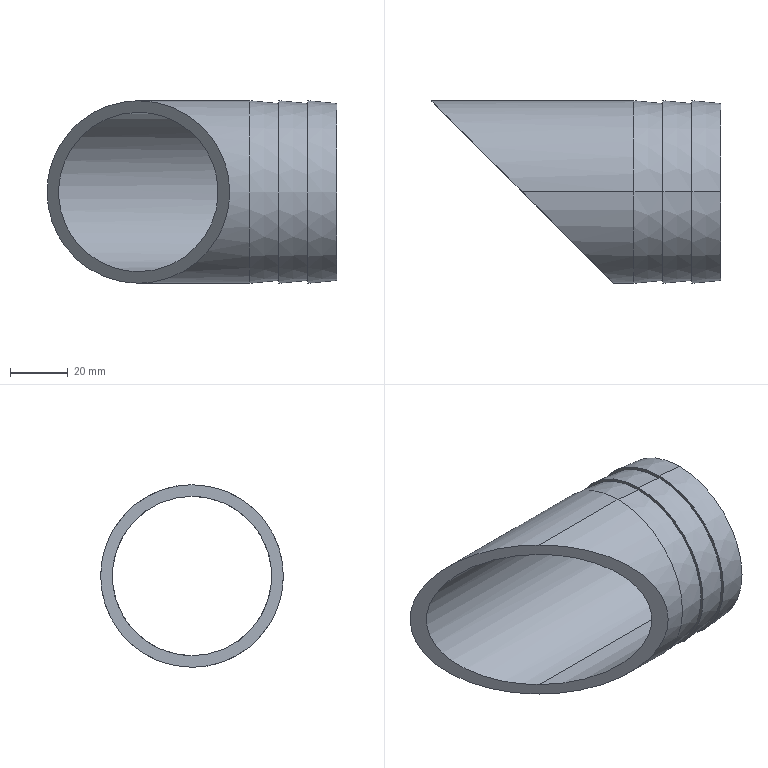Part | SolidWorks | features ICE 1, Revolution 1 | 1 solid | 14 faces | box 100 x 63 x 63 mm | volume 47848 mm3 | cone 6 | cylinder 4 | plane 4 | commonest cylinder face diameters 55 x2 63 x2
STEP:
#1=CARTESIAN_POINT('',(100.,0.,30.5));
#2=VERTEX_POINT('',#1);
#3=CARTESIAN_POINT('',(100.,0.,-30.5));
#4=VERTEX_POINT('',#3);
#5=CARTESIAN_POINT('',(100.,0.,0.));
#6=DIRECTION('',(-1.,0.,0.));
#7=DIRECTION('',(0.,0.,1.));
#8=AXIS2_PLACEMENT_3D('',#5,#6,#7);
#9=CIRCLE('',#8,30.5);
#10=EDGE_CURVE('',#2,#4,#9,.T.);
#11=ORIENTED_EDGE('',*,*,#10,.T.);
#12=CARTESIAN_POINT('',(90.,0.,-31.5));
#13=VERTEX_POINT('',#12);
#14=CARTESIAN_POINT('',(100.,0.,-30.5));
#15=DIRECTION('',(-0.995,0.,-0.0995));
#16=VECTOR('',#15,1000.);
#17=LINE('',#14,#16);
#18=EDGE_CURVE('',#4,#13,#17,.T.);
#19=ORIENTED_EDGE('',*,*,#18,.T.);
#20=CARTESIAN_POINT('',(90.,0.,31.5));
#21=VERTEX_POINT('',#20);
#22=CARTESIAN_POINT('',(90.,0.,0.));
#23=DIRECTION('',(-1.,0.,0.));
#24=DIRECTION('',(0.,0.,1.));
#25=AXIS2_PLACEMENT_3D('',#22,#23,#24);
#26=CIRCLE('',#25,31.5);
#27=EDGE_CURVE('',#21,#13,#26,.T.);
#28=ORIENTED_EDGE('',*,*,#27,.F.);
#29=CARTESIAN_POINT('',(100.,0.,30.5));
#30=DIRECTION('',(-0.995,0.,0.0995));
#31=VECTOR('',#30,1000.);
#32=LINE('',#29,#31);
#33=EDGE_CURVE('',#2,#21,#32,.T.);
#34=ORIENTED_EDGE('',*,*,#33,.F.);
#35=EDGE_LOOP('',(#11,#19,#28,#34));
#36=FACE_OUTER_BOUND('',#35,.T.);
#37=CARTESIAN_POINT('',(100.,0.,0.));
#38=DIRECTION('',(-1.,0.,0.));
#39=DIRECTION('',(0.,0.,1.));
#40=AXIS2_PLACEMENT_3D('',#37,#38,#39);
#41=CONICAL_SURFACE('',#40,30.5,0.09967);
#42=ADVANCED_FACE('',(#36),#41,.T.);
#43=CARTESIAN_POINT('',(90.,0.,30.5));
#44=VERTEX_POINT('',#43);
#45=CARTESIAN_POINT('',(90.,0.,-30.5));
#46=VERTEX_POINT('',#45);
#47=CARTESIAN_POINT('',(90.,0.,0.));
#48=DIRECTION('',(-1.,0.,0.));
#49=DIRECTION('',(0.,0.,1.));
#50=AXIS2_PLACEMENT_3D('',#47,#48,#49);
#51=CIRCLE('',#50,30.5);
#52=EDGE_CURVE('',#44,#46,#51,.T.);
#53=ORIENTED_EDGE('',*,*,#52,.T.);
#54=CARTESIAN_POINT('',(80.,0.,-31.5));
#55=VERTEX_POINT('',#54);
#56=CARTESIAN_POINT('',(90.,0.,-30.5));
#57=DIRECTION('',(-0.995,0.,-0.0995));
#58=VECTOR('',#57,1000.);
#59=LINE('',#56,#58);
#60=EDGE_CURVE('',#46,#55,#59,.T.);
#61=ORIENTED_EDGE('',*,*,#60,.T.);
#62=CARTESIAN_POINT('',(80.,0.,31.5));
#63=VERTEX_POINT('',#62);
#64=CARTESIAN_POINT('',(80.,0.,0.));
#65=DIRECTION('',(-1.,0.,0.));
#66=DIRECTION('',(0.,0.,1.));
#67=AXIS2_PLACEMENT_3D('',#64,#65,#66);
#68=CIRCLE('',#67,31.5);
#69=EDGE_CURVE('',#63,#55,#68,.T.);
#70=ORIENTED_EDGE('',*,*,#69,.F.);
#71=CARTESIAN_POINT('',(90.,0.,30.5));
#72=DIRECTION('',(-0.995,0.,0.0995));
#73=VECTOR('',#72,1000.);
#74=LINE('',#71,#73);
#75=EDGE_CURVE('',#44,#63,#74,.T.);
#76=ORIENTED_EDGE('',*,*,#75,.F.);
#77=EDGE_LOOP('',(#53,#61,#70,#76));
#78=FACE_OUTER_BOUND('',#77,.T.);
#79=CARTESIAN_POINT('',(90.,0.,0.));
#80=DIRECTION('',(-1.,0.,0.));
#81=DIRECTION('',(0.,0.,1.));
#82=AXIS2_PLACEMENT_3D('',#79,#80,#81);
#83=CONICAL_SURFACE('',#82,30.5,0.09967);
#84=ADVANCED_FACE('',(#78),#83,.T.);
#85=CARTESIAN_POINT('',(80.,0.,30.5));
#86=VERTEX_POINT('',#85);
#87=CARTESIAN_POINT('',(80.,0.,-30.5));
#88=VERTEX_POINT('',#87);
#89=CARTESIAN_POINT('',(80.,0.,0.));
#90=DIRECTION('',(-1.,0.,0.));
#91=DIRECTION('',(0.,0.,1.));
#92=AXIS2_PLACEMENT_3D('',#89,#90,#91);
#93=CIRCLE('',#92,30.5);
#94=EDGE_CURVE('',#86,#88,#93,.T.);
#95=ORIENTED_EDGE('',*,*,#94,.T.);
#96=CARTESIAN_POINT('',(70.,0.,-31.5));
#97=VERTEX_POINT('',#96);
#98=CARTESIAN_POINT('',(80.,0.,-30.5));
#99=DIRECTION('',(-0.995,0.,-0.0995));
#100=VECTOR('',#99,1000.);
#101=LINE('',#98,#100);
#102=EDGE_CURVE('',#88,#97,#101,.T.);
#103=ORIENTED_EDGE('',*,*,#102,.T.);
#104=CARTESIAN_POINT('',(70.,0.,31.5));
#105=VERTEX_POINT('',#104);
#106=CARTESIAN_POINT('',(70.,0.,0.));
#107=DIRECTION('',(-1.,0.,0.));
#108=DIRECTION('',(0.,0.,1.));
#109=AXIS2_PLACEMENT_3D('',#106,#107,#108);
#110=CIRCLE('',#109,31.5);
#111=EDGE_CURVE('',#105,#97,#110,.T.);
#112=ORIENTED_EDGE('',*,*,#111,.F.);
#113=CARTESIAN_POINT('',(80.,0.,30.5));
#114=DIRECTION('',(-0.995,0.,0.0995));
#115=VECTOR('',#114,1000.);
#116=LINE('',#113,#115);
#117=EDGE_CURVE('',#86,#105,#116,.T.);
#118=ORIENTED_EDGE('',*,*,#117,.F.);
#119=EDGE_LOOP('',(#95,#103,#112,#118));
#120=FACE_OUTER_BOUND('',#119,.T.);
#121=CARTESIAN_POINT('',(80.,0.,0.));
#122=DIRECTION('',(-1.,0.,0.));
#123=DIRECTION('',(0.,0.,1.));
#124=AXIS2_PLACEMENT_3D('',#121,#122,#123);
#125=CONICAL_SURFACE('',#124,30.5,0.09967);
#126=ADVANCED_FACE('',(#120),#125,.T.);
#127=ORIENTED_EDGE('',*,*,#111,.T.);
#128=CARTESIAN_POINT('',(31.5,0.,-31.5));
#129=VERTEX_POINT('',#128);
#130=CARTESIAN_POINT('',(0.,0.,-31.5));
#131=DIRECTION('',(-1.,0.,0.));
#132=VECTOR('',#131,1000.);
#133=LINE('',#130,#132);
#134=EDGE_CURVE('',#97,#129,#133,.T.);
#135=ORIENTED_EDGE('',*,*,#134,.T.);
#136=CARTESIAN_POINT('',(31.5,0.,31.5));
#137=VERTEX_POINT('',#136);
#138=CARTESIAN_POINT('',(31.5,0.,-31.5));
#139=CARTESIAN_POINT('',(-31.5,63.,-31.5));
#140=CARTESIAN_POINT('',(-31.5,63.,31.5));
#141=CARTESIAN_POINT('',(31.5,0.,31.5));
#142=(BOUNDED_CURVE()B_SPLINE_CURVE(3,(#138,#139,#140,#141),.UNSPECIFIED.,.F.,.F.)B_SPLINE_CURVE_WITH_KNOTS((4,4),(4.712,7.854),.UNSPECIFIED.)CURVE()GEOMETRIC_REPRESENTATION_ITEM()RATIONAL_B_SPLINE_CURVE((1.,0.3333,0.3333,1.))REPRESENTATION_ITEM(''));
#143=EDGE_CURVE('',#129,#137,#142,.T.);
#144=ORIENTED_EDGE('',*,*,#143,.T.);
#145=CARTESIAN_POINT('',(0.,0.,31.5));
#146=DIRECTION('',(-1.,0.,0.));
#147=VECTOR('',#146,1000.);
#148=LINE('',#145,#147);
#149=EDGE_CURVE('',#105,#137,#148,.T.);
#150=ORIENTED_EDGE('',*,*,#149,.F.);
#151=EDGE_LOOP('',(#127,#135,#144,#150));
#152=FACE_OUTER_BOUND('',#151,.T.);
#153=CARTESIAN_POINT('',(0.,0.,0.));
#154=DIRECTION('',(-1.,0.,0.));
#155=DIRECTION('',(0.,0.,1.));
#156=AXIS2_PLACEMENT_3D('',#153,#154,#155);
#157=CYLINDRICAL_SURFACE('',#156,31.5);
#158=ADVANCED_FACE('',(#152),#157,.T.);
#159=CARTESIAN_POINT('',(100.,0.,-27.5));
#160=VERTEX_POINT('',#159);
#161=CARTESIAN_POINT('',(100.,0.,27.5));
#162=VERTEX_POINT('',#161);
#163=CARTESIAN_POINT('',(100.,0.,0.));
#164=DIRECTION('',(-1.,0.,0.));
#165=DIRECTION('',(0.,0.,1.));
#166=AXIS2_PLACEMENT_3D('',#163,#164,#165);
#167=CIRCLE('',#166,27.5);
#168=EDGE_CURVE('',#160,#162,#167,.T.);
#169=ORIENTED_EDGE('',*,*,#168,.F.);
#170=CARTESIAN_POINT('',(31.5,0.,-27.5));
#171=VERTEX_POINT('',#170);
#172=CARTESIAN_POINT('',(0.,0.,-27.5));
#173=DIRECTION('',(-1.,0.,0.));
#174=VECTOR('',#173,1000.);
#175=LINE('',#172,#174);
#176=EDGE_CURVE('',#160,#171,#175,.T.);
#177=ORIENTED_EDGE('',*,*,#176,.T.);
#178=CARTESIAN_POINT('',(31.5,0.,27.5));
#179=VERTEX_POINT('',#178);
#180=CARTESIAN_POINT('',(31.5,0.,-27.5));
#181=CARTESIAN_POINT('',(86.5,-55.,-27.5));
#182=CARTESIAN_POINT('',(86.5,-55.,27.5));
#183=CARTESIAN_POINT('',(31.5,0.,27.5));
#184=(BOUNDED_CURVE()B_SPLINE_CURVE(3,(#180,#181,#182,#183),.UNSPECIFIED.,.F.,.F.)B_SPLINE_CURVE_WITH_KNOTS((4,4),(1.571,4.712),.UNSPECIFIED.)CURVE()GEOMETRIC_REPRESENTATION_ITEM()RATIONAL_B_SPLINE_CURVE((1.,0.3333,0.3333,1.))REPRESENTATION_ITEM(''));
#185=EDGE_CURVE('',#171,#179,#184,.T.);
#186=ORIENTED_EDGE('',*,*,#185,.T.);
#187=CARTESIAN_POINT('',(0.,0.,27.5));
#188=DIRECTION('',(-1.,0.,0.));
#189=VECTOR('',#188,1000.);
#190=LINE('',#187,#189);
#191=EDGE_CURVE('',#162,#179,#190,.T.);
#192=ORIENTED_EDGE('',*,*,#191,.F.);
#193=EDGE_LOOP('',(#169,#177,#186,#192));
#194=FACE_OUTER_BOUND('',#193,.T.);
#195=CARTESIAN_POINT('',(0.,0.,0.));
#196=DIRECTION('',(-1.,0.,0.));
#197=DIRECTION('',(0.,0.,1.));
#198=AXIS2_PLACEMENT_3D('',#195,#196,#197);
#199=CYLINDRICAL_SURFACE('',#198,27.5);
#200=ADVANCED_FACE('',(#194),#199,.F.);
#201=ORIENTED_EDGE('',*,*,#10,.F.);
#202=CARTESIAN_POINT('',(100.,0.,0.));
#203=DIRECTION('',(-1.,0.,0.));
#204=DIRECTION('',(0.,0.,1.));
#205=AXIS2_PLACEMENT_3D('',#202,#203,#204);
#206=CIRCLE('',#205,30.5);
#207=EDGE_CURVE('',#4,#2,#206,.T.);
#208=ORIENTED_EDGE('',*,*,#207,.F.);
#209=EDGE_LOOP('',(#201,#208));
#210=FACE_OUTER_BOUND('',#209,.T.);
#211=CARTESIAN_POINT('',(100.,0.,0.));
#212=DIRECTION('',(-1.,0.,0.));
#213=DIRECTION('',(0.,0.,1.));
#214=AXIS2_PLACEMENT_3D('',#211,#212,#213);
#215=CIRCLE('',#214,27.5);
#216=EDGE_CURVE('',#162,#160,#215,.T.);
#217=ORIENTED_EDGE('',*,*,#216,.T.);
#218=ORIENTED_EDGE('',*,*,#168,.T.);
#219=EDGE_LOOP('',(#217,#218));
#220=FACE_BOUND('',#219,.T.);
#221=CARTESIAN_POINT('',(100.,30.5,0.));
#222=DIRECTION('',(-1.,0.,0.));
#223=DIRECTION('',(0.,0.,1.));
#224=AXIS2_PLACEMENT_3D('',#221,#222,#223);
#225=PLANE('',#224);
#226=ADVANCED_FACE('',(#210,#220),#225,.F.);
#227=ORIENTED_EDGE('',*,*,#176,.F.);
#228=ORIENTED_EDGE('',*,*,#216,.F.);
#229=ORIENTED_EDGE('',*,*,#191,.T.);
#230=CARTESIAN_POINT('',(31.5,0.,27.5));
#231=CARTESIAN_POINT('',(-23.5,55.,27.5));
#232=CARTESIAN_POINT('',(-23.5,55.,-27.5));
#233=CARTESIAN_POINT('',(31.5,0.,-27.5));
#234=(BOUNDED_CURVE()B_SPLINE_CURVE(3,(#230,#231,#232,#233),.UNSPECIFIED.,.F.,.F.)B_SPLINE_CURVE_WITH_KNOTS((4,4),(4.712,7.854),.UNSPECIFIED.)CURVE()GEOMETRIC_REPRESENTATION_ITEM()RATIONAL_B_SPLINE_CURVE((1.,0.3333,0.3333,1.))REPRESENTATION_ITEM(''));
#235=EDGE_CURVE('',#179,#171,#234,.T.);
#236=ORIENTED_EDGE('',*,*,#235,.T.);
#237=EDGE_LOOP('',(#227,#228,#229,#236));
#238=FACE_OUTER_BOUND('',#237,.T.);
#239=CARTESIAN_POINT('',(0.,0.,0.));
#240=DIRECTION('',(-1.,0.,0.));
#241=DIRECTION('',(0.,0.,1.));
#242=AXIS2_PLACEMENT_3D('',#239,#240,#241);
#243=CYLINDRICAL_SURFACE('',#242,27.5);
#244=ADVANCED_FACE('',(#238),#243,.F.);
#245=ORIENTED_EDGE('',*,*,#134,.F.);
#246=CARTESIAN_POINT('',(70.,0.,0.));
#247=DIRECTION('',(-1.,0.,0.));
#248=DIRECTION('',(0.,0.,1.));
#249=AXIS2_PLACEMENT_3D('',#246,#247,#248);
#250=CIRCLE('',#249,31.5);
#251=EDGE_CURVE('',#97,#105,#250,.T.);
#252=ORIENTED_EDGE('',*,*,#251,.T.);
#253=ORIENTED_EDGE('',*,*,#149,.T.);
#254=CARTESIAN_POINT('',(31.5,0.,31.5));
#255=CARTESIAN_POINT('',(94.5,-63.,31.5));
#256=CARTESIAN_POINT('',(94.5,-63.,-31.5));
#257=CARTESIAN_POINT('',(31.5,0.,-31.5));
#258=(BOUNDED_CURVE()B_SPLINE_CURVE(3,(#254,#255,#256,#257),.UNSPECIFIED.,.F.,.F.)B_SPLINE_CURVE_WITH_KNOTS((4,4),(1.571,4.712),.UNSPECIFIED.)CURVE()GEOMETRIC_REPRESENTATION_ITEM()RATIONAL_B_SPLINE_CURVE((1.,0.3333,0.3333,1.))REPRESENTATION_ITEM(''));
#259=EDGE_CURVE('',#137,#129,#258,.T.);
#260=ORIENTED_EDGE('',*,*,#259,.T.);
#261=EDGE_LOOP('',(#245,#252,#253,#260));
#262=FACE_OUTER_BOUND('',#261,.T.);
#263=CARTESIAN_POINT('',(0.,0.,0.));
#264=DIRECTION('',(-1.,0.,0.));
#265=DIRECTION('',(0.,0.,1.));
#266=AXIS2_PLACEMENT_3D('',#263,#264,#265);
#267=CYLINDRICAL_SURFACE('',#266,31.5);
#268=ADVANCED_FACE('',(#262),#267,.T.);
#269=ORIENTED_EDGE('',*,*,#102,.F.);
#270=CARTESIAN_POINT('',(80.,0.,0.));
#271=DIRECTION('',(-1.,0.,0.));
#272=DIRECTION('',(0.,0.,1.));
#273=AXIS2_PLACEMENT_3D('',#270,#271,#272);
#274=CIRCLE('',#273,30.5);
#275=EDGE_CURVE('',#88,#86,#274,.T.);
#276=ORIENTED_EDGE('',*,*,#275,.T.);
#277=ORIENTED_EDGE('',*,*,#117,.T.);
#278=ORIENTED_EDGE('',*,*,#251,.F.);
#279=EDGE_LOOP('',(#269,#276,#277,#278));
#280=FACE_OUTER_BOUND('',#279,.T.);
#281=CARTESIAN_POINT('',(80.,0.,0.));
#282=DIRECTION('',(-1.,0.,0.));
#283=DIRECTION('',(0.,0.,1.));
#284=AXIS2_PLACEMENT_3D('',#281,#282,#283);
#285=CONICAL_SURFACE('',#284,30.5,0.09967);
#286=ADVANCED_FACE('',(#280),#285,.T.);
#287=ORIENTED_EDGE('',*,*,#94,.F.);
#288=ORIENTED_EDGE('',*,*,#275,.F.);
#289=EDGE_LOOP('',(#287,#288));
#290=FACE_BOUND('',#289,.T.);
#291=ORIENTED_EDGE('',*,*,#69,.T.);
#292=CARTESIAN_POINT('',(80.,0.,0.));
#293=DIRECTION('',(-1.,0.,0.));
#294=DIRECTION('',(0.,0.,1.));
#295=AXIS2_PLACEMENT_3D('',#292,#293,#294);
#296=CIRCLE('',#295,31.5);
#297=EDGE_CURVE('',#55,#63,#296,.T.);
#298=ORIENTED_EDGE('',*,*,#297,.T.);
#299=EDGE_LOOP('',(#291,#298));
#300=FACE_OUTER_BOUND('',#299,.T.);
#301=CARTESIAN_POINT('',(80.,30.5,0.));
#302=DIRECTION('',(1.,0.,0.));
#303=DIRECTION('',(0.,0.,-1.));
#304=AXIS2_PLACEMENT_3D('',#301,#302,#303);
#305=PLANE('',#304);
#306=ADVANCED_FACE('',(#290,#300),#305,.F.);
#307=ORIENTED_EDGE('',*,*,#60,.F.);
#308=CARTESIAN_POINT('',(90.,0.,0.));
#309=DIRECTION('',(-1.,0.,0.));
#310=DIRECTION('',(0.,0.,1.));
#311=AXIS2_PLACEMENT_3D('',#308,#309,#310);
#312=CIRCLE('',#311,30.5);
#313=EDGE_CURVE('',#46,#44,#312,.T.);
#314=ORIENTED_EDGE('',*,*,#313,.T.);
#315=ORIENTED_EDGE('',*,*,#75,.T.);
#316=ORIENTED_EDGE('',*,*,#297,.F.);
#317=EDGE_LOOP('',(#307,#314,#315,#316));
#318=FACE_OUTER_BOUND('',#317,.T.);
#319=CARTESIAN_POINT('',(90.,0.,0.));
#320=DIRECTION('',(-1.,0.,0.));
#321=DIRECTION('',(0.,0.,1.));
#322=AXIS2_PLACEMENT_3D('',#319,#320,#321);
#323=CONICAL_SURFACE('',#322,30.5,0.09967);
#324=ADVANCED_FACE('',(#318),#323,.T.);
#325=ORIENTED_EDGE('',*,*,#52,.F.);
#326=ORIENTED_EDGE('',*,*,#313,.F.);
#327=EDGE_LOOP('',(#325,#326));
#328=FACE_BOUND('',#327,.T.);
#329=ORIENTED_EDGE('',*,*,#27,.T.);
#330=CARTESIAN_POINT('',(90.,0.,0.));
#331=DIRECTION('',(-1.,0.,0.));
#332=DIRECTION('',(0.,0.,1.));
#333=AXIS2_PLACEMENT_3D('',#330,#331,#332);
#334=CIRCLE('',#333,31.5);
#335=EDGE_CURVE('',#13,#21,#334,.T.);
#336=ORIENTED_EDGE('',*,*,#335,.T.);
#337=EDGE_LOOP('',(#329,#336));
#338=FACE_OUTER_BOUND('',#337,.T.);
#339=CARTESIAN_POINT('',(90.,30.5,0.));
#340=DIRECTION('',(1.,0.,0.));
#341=DIRECTION('',(0.,0.,-1.));
#342=AXIS2_PLACEMENT_3D('',#339,#340,#341);
#343=PLANE('',#342);
#344=ADVANCED_FACE('',(#328,#338),#343,.F.);
#345=ORIENTED_EDGE('',*,*,#18,.F.);
#346=ORIENTED_EDGE('',*,*,#207,.T.);
#347=ORIENTED_EDGE('',*,*,#33,.T.);
#348=ORIENTED_EDGE('',*,*,#335,.F.);
#349=EDGE_LOOP('',(#345,#346,#347,#348));
#350=FACE_OUTER_BOUND('',#349,.T.);
#351=CARTESIAN_POINT('',(100.,0.,0.));
#352=DIRECTION('',(-1.,0.,0.));
#353=DIRECTION('',(0.,0.,1.));
#354=AXIS2_PLACEMENT_3D('',#351,#352,#353);
#355=CONICAL_SURFACE('',#354,30.5,0.09967);
#356=ADVANCED_FACE('',(#350),#355,.T.);
#357=ORIENTED_EDGE('',*,*,#259,.F.);
#358=ORIENTED_EDGE('',*,*,#143,.F.);
#359=EDGE_LOOP('',(#357,#358));
#360=FACE_OUTER_BOUND('',#359,.T.);
#361=ORIENTED_EDGE('',*,*,#235,.F.);
#362=ORIENTED_EDGE('',*,*,#185,.F.);
#363=EDGE_LOOP('',(#361,#362));
#364=FACE_BOUND('',#363,.T.);
#365=CARTESIAN_POINT('',(0.,31.5,205.541));
#366=DIRECTION('',(0.7071,0.7071,0.));
#367=DIRECTION('',(-0.7071,0.7071,0.));
#368=AXIS2_PLACEMENT_3D('',#365,#366,#367);
#369=PLANE('',#368);
#370=ADVANCED_FACE('',(#360,#364),#369,.F.);
#371=CLOSED_SHELL('',(#42,#84,#126,#158,#200,#226,#244,#268,#286,#306,#324,#344,#356,#370));
#372=MANIFOLD_SOLID_BREP('',#371);
#373=CARTESIAN_POINT('',(0.,0.,0.));
#374=DIRECTION('',(0.,0.,1.));
#375=DIRECTION('',(1.,0.,0.));
#376=AXIS2_PLACEMENT_3D('',#373,#374,#375);
#377=(LENGTH_UNIT()NAMED_UNIT(*)SI_UNIT(.MILLI.,.METRE.));
#378=UNCERTAINTY_MEASURE_WITH_UNIT(LENGTH_MEASURE(0.00001),#377,'','');
#379=(NAMED_UNIT(*)PLANE_ANGLE_UNIT()SI_UNIT($,.RADIAN.));
#380=(NAMED_UNIT(*)SI_UNIT($,.STERADIAN.)SOLID_ANGLE_UNIT());
#381=(GEOMETRIC_REPRESENTATION_CONTEXT(3)GLOBAL_UNCERTAINTY_ASSIGNED_CONTEXT((#378))GLOBAL_UNIT_ASSIGNED_CONTEXT((#377,#379,#380))REPRESENTATION_CONTEXT('',''));
#382=ADVANCED_BREP_SHAPE_REPRESENTATION('',(#372,#376),#381);